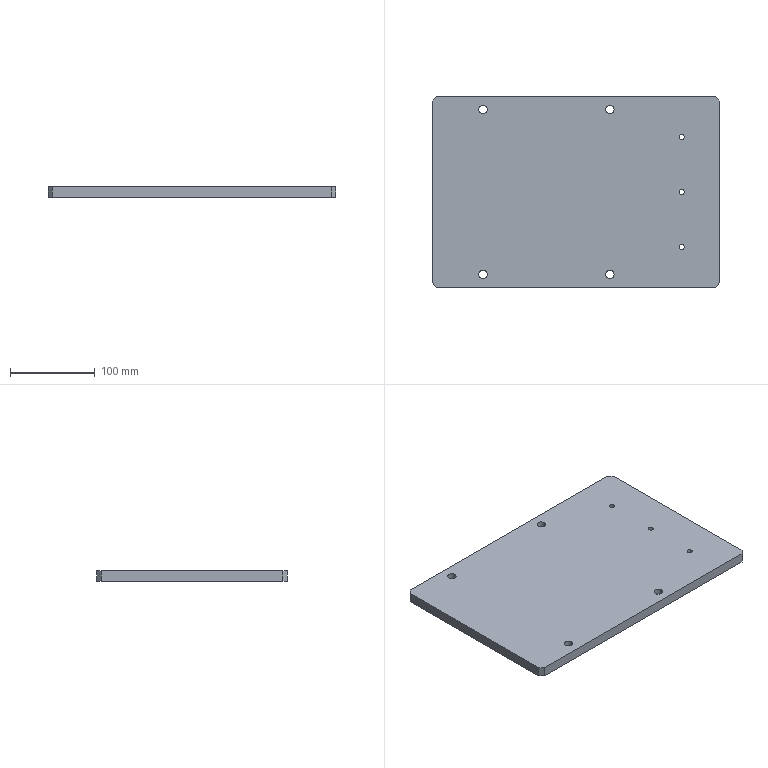Part | STEP file | MOTOR.PLATE.1.stp | 1 solid | 24 faces | box 340 x 225 x 12 mm | volume 912612 mm3 | spline 10 | cylinder 8 | plane 6 | commonest cylinder face diameters 6 x4 10 x4